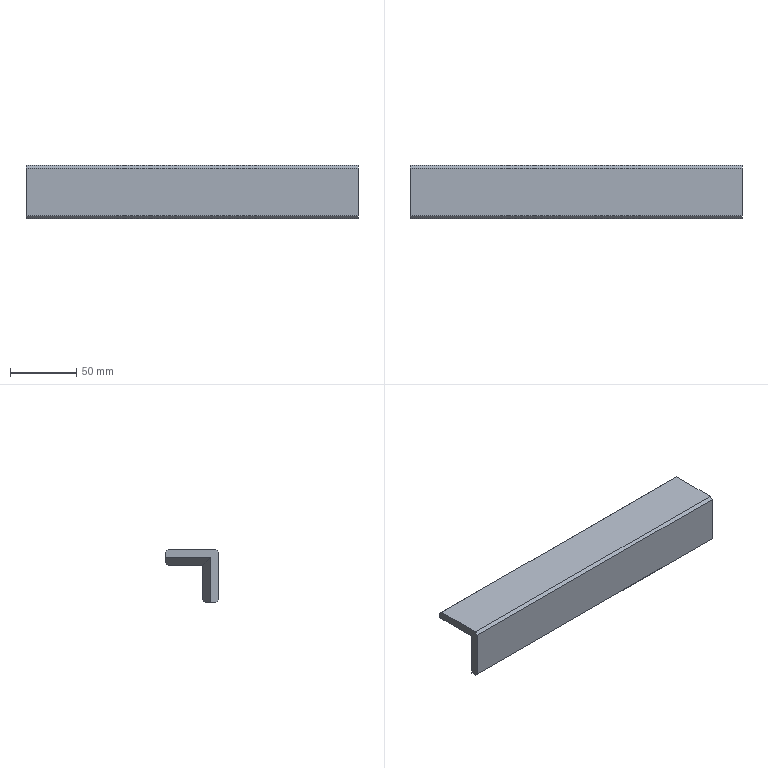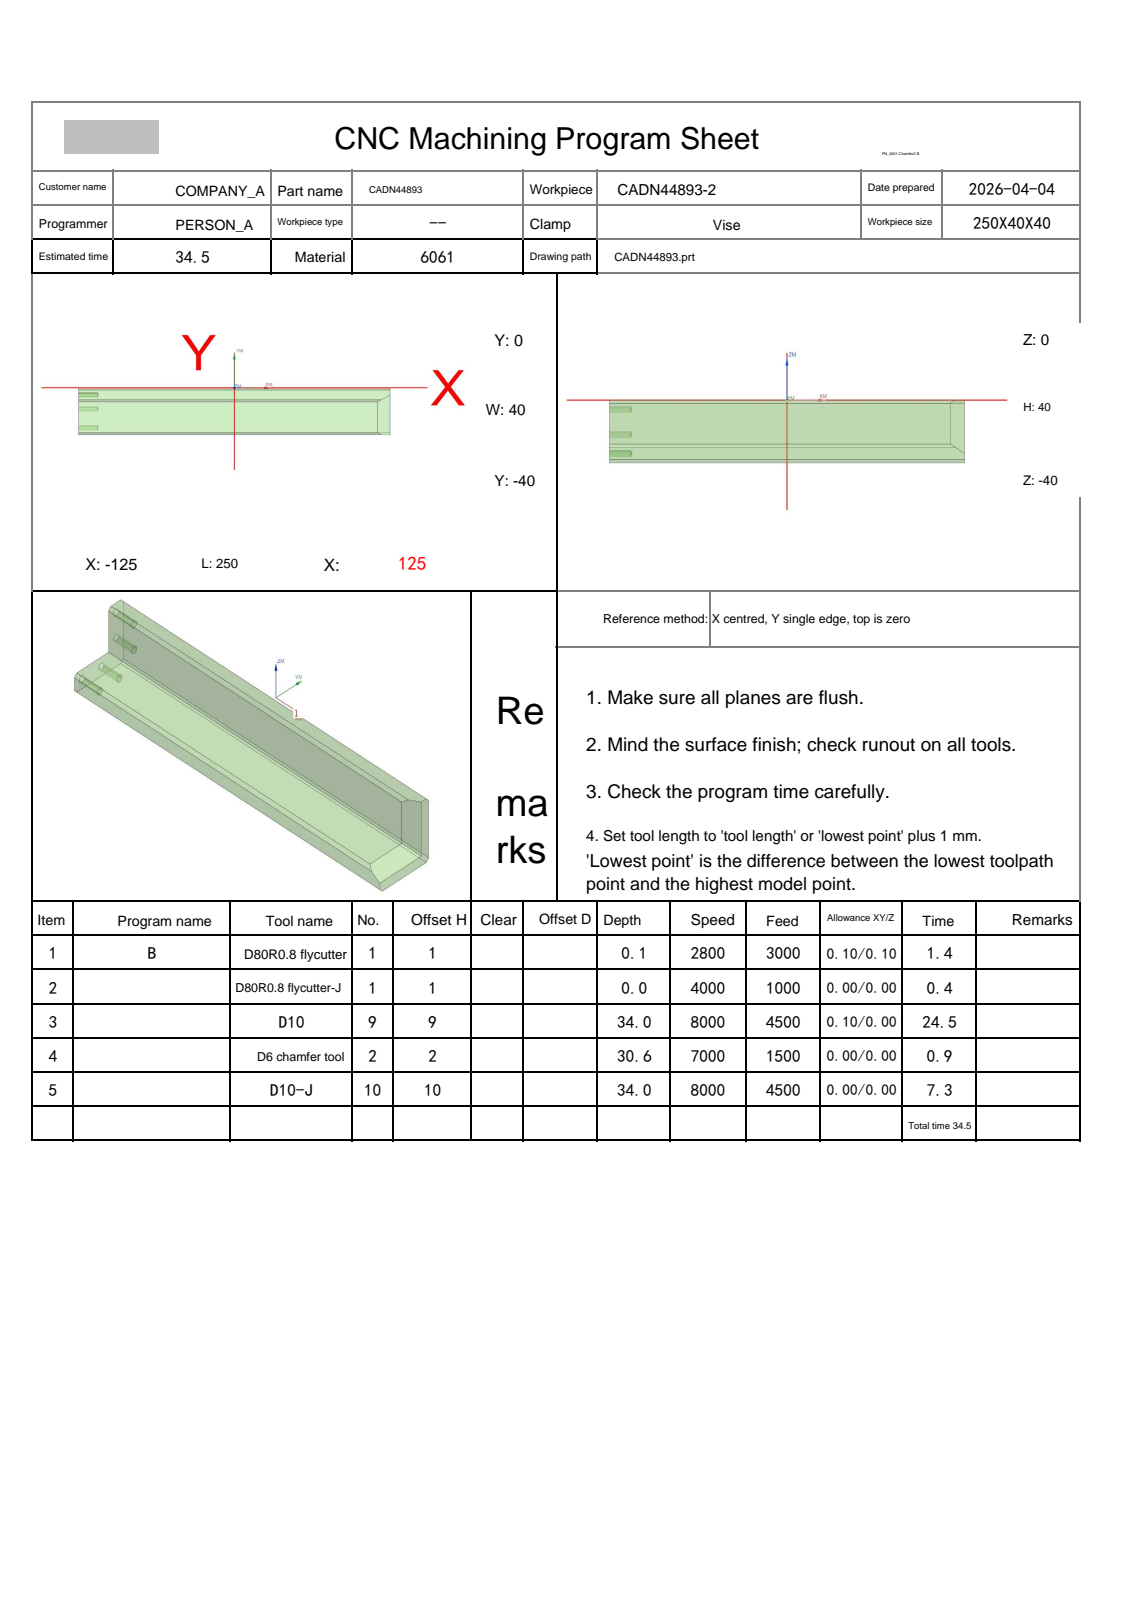NC program | NX | posted by the shop | part box 250 x 40 x 40 mm
Lines 109 to 1286 of 8932:
N3 T09 M06
(D10  D=10. R=0. H=09 ce=0.10 di=0.10)
G00 G90 G54 X8.423 Y-52.151 M03 S8000
G43 H09 Z14.5
M08
Z.702
G01 Z-.498 F4000.
Y-50.
G03 X1.423 Y-43. I-7. J0.0
G01 X-125.08
Y-42.864
Y-17.796
Y-17.039
Y-16.914
Y-15.638
X-118.08 Y-15.64
X117.385
G03 X120.127 Y-14.871 I-.016 J5.333
G01 X127.977 Y-10.161
G03 X129.233 Y-8.844 I-3.041 J4.158
X130.051 Y-6.704 I-4.233 J2.844
G01 X130.074 Y-6.707
X130.147 Y-6.712
X130.131 Y-6.784
Y-9.994
G02 X128.804 Y-11.291 I-5.196 J3.991
G01 X128.698 Y-11.362
X128. Y-11.78
Y-40.08
X123.457
X123.382 Y-40.73
G02 X122.477 Y-43. I-5.03 J.691
G01 X-.563
G02 X-1.375 Y-42.582 I.001 J1.
G01 X-5.778 Y-36.418
G03 X-6.591 Y-36. I-.813 J-.582
G01 X-117.083
G02 X-118.08 Y-35.003 I.003 J1.
G01 Y-23.636
G02 X-117.083 Y-22.64 I1. J-.003
G01 X117.396
G03 X119.806 Y-22.397 I-.026 J12.333
G01 X120. Y-22.378
G02 X121. Y-23.374 I0.0 J-1.
G01 Y-32.868
G02 X120.435 Y-33.765 I-1. J.003
G03 X118.047 Y-35.637 I3.022 J-6.314
G02 X117.279 Y-36. I-.771 J.637
G01 X-.913
G02 X-1.619 Y-35.708 I.001 J1.
G01 X-5.534 Y-31.793
G03 X-6.241 Y-31.5 I-.707 J-.707
G01 X-112.584
G02 X-113.58 Y-30.504 I.004 J1.
G01 Y-28.136
G02 X-112.584 Y-27.14 I1. J-.004
G01 X115.504
G02 X116.5 Y-28.136 I-.004 J-1.
G01 Y-30.443
G02 X116.139 Y-31.208 I-1. J.004
G01 X116.066 Y-31.269
G02 X115.43 Y-31.5 I-.639 J.769
G01 X-3.577
X-4.077
G03 X-11.077 Y-38.5 I0.0 J-7.
G01 Y-52.151
Z.702
G00 Z3.
G01 X8.423 F6000.
G00 Z.204
G01 Z-.996 F4000.
Y-50.
G03 X1.423 Y-43. I-7. J0.0
G01 X-125.08
Y-42.864
Y-17.796
Y-17.099
Y-16.914
Y-16.136
X-118.08 Y-16.138
X116.372
X116.447
G03 X119.297 Y-15.37 I0.0 J5.664
G01 X119.698 Y-15.129
X120.127 Y-14.871
X127.625 Y-10.373
X127.977 Y-10.161
G03 X129.233 Y-8.844 I-3.041 J4.158
X130.051 Y-6.704 I-4.233 J2.844
G01 X130.074 Y-6.707
X130.147 Y-6.712
X130.131 Y-6.784
Y-9.994
G02 X128.804 Y-11.291 I-5.196 J3.991
G01 X128.698 Y-11.362
X128.344 Y-11.574
X128. Y-11.78
Y-40.08
X123.457
X123.382 Y-40.73
G02 X122.477 Y-43. I-5.03 J.691
G01 X-3.577
G02 X-4.548 Y-42.238 I0.0 J1.
G01 X-5.89 Y-36.761
G03 X-6.86 Y-36. I-.971 J-.239
G01 X-117.083
G02 X-118.08 Y-35.004 I.004 J1.
G01 Y-24.134
G02 X-117.084 Y-23.138 I1. J-.004
G01 X116.334
X116.447
G03 X119.743 Y-22.702 I0.0 J12.664
G02 X120. Y-22.668 I.257 J-.967
X121. Y-23.665 I0.0 J-1.
G01 Y-32.869
G02 X120.435 Y-33.765 I-1. J.004
G03 X118.046 Y-35.638 I3.021 J-6.314
G02 X117.28 Y-36. I-.77 J.638
G01 X-.913
G02 X-1.619 Y-35.708 I.001 J1.
G01 X-5.534 Y-31.793
G03 X-6.241 Y-31.5 I-.707 J-.707
G01 X-112.584
G02 X-113.58 Y-30.504 I.004 J1.
G01 Y-28.634
G02 X-112.584 Y-27.638 I1. J-.004
G01 X115.504
G02 X116.5 Y-28.634 I-.004 J-1.
G01 Y-30.443
G02 X116.14 Y-31.208 I-1. J.004
G01 X116.066 Y-31.269
G02 X115.431 Y-31.5 I-.639 J.769
G01 X-3.577
X-4.077
G03 X-11.077 Y-38.5 I0.0 J-7.
G01 Y-52.151
Z.204
G00 Z2.502
G01 X8.423 F6000.
G00 Z-.295
G01 Z-1.495 F4000.
Y-50.
G03 X1.423 Y-43. I-7. J0.0
G01 X-125.08
Y-42.864
Y-17.796
Y-17.099
Y-16.914
Y-16.634
X-118.08 Y-16.636
X115.724
G03 X118.466 Y-15.868 I-.016 J5.333
G01 X127.625 Y-10.373
X127.977 Y-10.161
G03 X129.233 Y-8.844 I-3.041 J4.158
X130.051 Y-6.704 I-4.233 J2.844
G01 X130.074 Y-6.707
X130.147 Y-6.712
X130.131 Y-6.784
Y-9.994
G02 X128.804 Y-11.291 I-5.196 J3.991
G01 X128.698 Y-11.362
X128. Y-11.78
Y-40.08
X123.457
X123.382 Y-40.73
G02 X122.477 Y-43. I-5.03 J.691
G01 X-3.577
G02 X-4.548 Y-42.238 I0.0 J1.
G01 X-5.89 Y-36.761
G03 X-6.86 Y-36. I-.971 J-.239
G01 X-117.084
G02 X-118.08 Y-35.004 I.004 J1.
G01 Y-24.632
G02 X-117.084 Y-23.636 I1. J-.004
G01 X115.735
G03 X119.682 Y-22.979 I-.026 J12.333
G02 X120. Y-22.927 I.318 J-.948
X121. Y-23.923 I0.0 J-1.
G01 Y-32.869
G02 X120.435 Y-33.765 I-1. J.004
G03 X118.046 Y-35.638 I3.021 J-6.314
G02 X117.28 Y-36. I-.77 J.638
G01 X-.913
G02 X-1.619 Y-35.708 I.001 J1.
G01 X-5.534 Y-31.793
G03 X-6.241 Y-31.5 I-.707 J-.707
G01 X-112.584
G02 X-113.58 Y-30.505 I.005 J1.
G01 Y-29.132
G02 X-112.584 Y-28.136 I1. J-.005
G01 X115.505
G02 X116.5 Y-29.132 I-.005 J-1.
G01 Y-30.443
G02 X116.14 Y-31.207 I-1. J.005
G01 X116.066 Y-31.269
G02 X115.431 Y-31.5 I-.639 J.769
G01 X-3.577
X-4.077
G03 X-11.077 Y-38.5 I0.0 J-7.
G01 Y-52.151
Z-.295
G00 Z2.004
G01 X8.423 F6000.
G00 Z-.793
G01 Z-1.993 F4000.
Y-50.
G03 X1.423 Y-43. I-7. J0.0
G01 X-125.08
Y-42.864
Y-18.499
Y-17.796
Y-17.099
X-118.08 Y-17.1
X115.
G03 X117.636 Y-16.366 I-.006 J5.125
G01 X118.466 Y-15.868
X127.625 Y-10.373
X127.977 Y-10.161
G03 X129.233 Y-8.844 I-3.041 J4.158
X130.051 Y-6.704 I-4.233 J2.844
G01 X130.074 Y-6.707
X130.147 Y-6.712
X130.131 Y-6.784
Y-9.994
G02 X128.804 Y-11.291 I-5.196 J3.991
G01 X128.698 Y-11.362
X128.344 Y-11.574
X128. Y-11.78
Y-40.08
X123.457
X123.382 Y-40.73
G02 X122.477 Y-43. I-5.03 J.691
G01 X-3.577
G02 X-4.548 Y-42.238 I0.0 J1.
G01 X-5.89 Y-36.761
G03 X-6.86 Y-36. I-.971 J-.239
G01 X-117.084
G02 X-118.08 Y-35.004 I.004 J1.
G01 Y-25.095
G02 X-117.084 Y-24.1 I1. J-.004
G01 X115.004
G03 X119.622 Y-23.181 I-.011 J12.125
G02 X120. Y-23.107 I.378 J-.926
X121. Y-24.103 I0.0 J-1.
G01 Y-32.869
G02 X120.436 Y-33.765 I-1. J.004
G03 X118.046 Y-35.638 I3.021 J-6.315
G02 X117.28 Y-36. I-.77 J.638
G01 X-.913
G02 X-1.619 Y-35.708 I.001 J1.
G01 X-5.534 Y-31.793
G03 X-6.241 Y-31.5 I-.707 J-.707
G01 X-112.585
G02 X-113.58 Y-30.505 I.005 J1.
G01 Y-29.595
G02 X-112.585 Y-28.6 I1. J-.005
G01 X115.008
G03 X115.476 Y-28.593 I-.015 J16.625
G01 X115.5 Y-28.592
G02 X116.5 Y-29.588 I0.0 J-1.
G01 Y-30.444
G02 X116.14 Y-31.207 I-1. J.005
G01 X116.065 Y-31.269
G02 X115.431 Y-31.5 I-.639 J.769
G01 X-3.577
X-4.077
G03 X-11.077 Y-38.5 I0.0 J-7.
G01 Y-52.151
Z-.793
G00 Z1.505
G01 X8.423 F6000.
G00 Z-1.291
G01 Z-2.491 F4000.
Y-50.
G03 X1.423 Y-43. I-7. J0.0
G01 X-125.08
Y-42.864
Y-18.5
Y-17.796
Y-17.099
X-118.08 Y-17.1
X115.
G03 X116.948 Y-16.713 I0.0 J5.1
X117.636 Y-16.366 I-1.948 J4.713
G01 X118.126 Y-16.072
X118.466 Y-15.868
X127.625 Y-10.372
X127.977 Y-10.161
G03 X129.233 Y-8.844 I-3.041 J4.158
X130.051 Y-6.704 I-4.233 J2.844
G01 X130.074 Y-6.707
X130.147 Y-6.712
X130.131 Y-6.784
Y-9.994
G02 X128.804 Y-11.291 I-5.196 J3.991
G01 X128.698 Y-11.362
X128.344 Y-11.574
X128. Y-11.78
Y-40.08
X123.457
X123.382 Y-40.73
G02 X122.477 Y-43. I-5.03 J.691
G01 X-3.577
G02 X-4.548 Y-42.238 I0.0 J1.
G01 X-5.89 Y-36.761
G03 X-6.86 Y-36. I-.971 J-.239
G01 X-117.084
G02 X-118.08 Y-35.005 I.005 J1.
G01 Y-25.095
G02 X-117.084 Y-24.1 I1. J-.005
G01 X115.
G03 X119.622 Y-23.182 I0.0 J12.1
G02 X120. Y-23.108 I.378 J-.926
X121. Y-24.104 I0.0 J-1.
G01 Y-32.869
G02 X120.436 Y-33.765 I-1. J.005
G03 X118.046 Y-35.638 I3.021 J-6.315
G02 X117.281 Y-36. I-.77 J.638
G01 X-.913
G02 X-1.619 Y-35.708 I.001 J1.
G01 X-5.534 Y-31.793
G03 X-6.241 Y-31.5 I-.707 J-.707
G01 X-112.585
G02 X-113.58 Y-30.505 I.005 J1.
G01 Y-29.595
G02 X-112.585 Y-28.6 I1. J-.005
G01 X115.
G03 X115.476 Y-28.593 I0.0 J16.6
G01 X115.5
G02 X116.5 Y-29.588 I0.0 J-1.
G01 Y-30.444
G02 X116.14 Y-31.207 I-1. J.005
G01 X116.065 Y-31.269
G02 X115.432 Y-31.5 I-.639 J.769
G01 X-3.577
X-4.077
G03 X-11.077 Y-38.5 I0.0 J-7.
G01 Y-52.151
Z-1.291
G00 Z1.007
G01 X8.423 F6000.
G00 Z-1.789
G01 Z-2.989 F4000.
Y-50.
G03 X1.423 Y-43. I-7. J0.0
G01 X-125.08
Y-42.864
Y-18.5
Y-17.796
Y-17.099
X-118.08 Y-17.1
X115.
G03 X116.948 Y-16.713 I0.0 J5.1
X117.636 Y-16.366 I-1.948 J4.713
G01 X118.466 Y-15.868
X118.857 Y-15.633
X119.249 Y-15.398
X127.626 Y-10.372
X127.977 Y-10.161
G03 X129.233 Y-8.844 I-3.041 J4.158
X130.051 Y-6.704 I-4.233 J2.844
G01 X130.074 Y-6.707
X130.147 Y-6.712
X130.131 Y-6.784
Y-9.994
G02 X128.804 Y-11.291 I-5.196 J3.991
G01 X128.698 Y-11.362
X128.344 Y-11.574
X128. Y-11.78
Y-40.08
X123.457
X123.382 Y-40.73
G02 X122.477 Y-43. I-5.03 J.691
G01 X-3.577
G02 X-4.548 Y-42.238 I0.0 J1.
G01 X-5.89 Y-36.761
G03 X-6.86 Y-36. I-.971 J-.239
G01 X-117.085
G02 X-118.08 Y-35.005 I.005 J1.
G01 Y-25.095
G02 X-117.085 Y-24.1 I1. J-.005
G01 X115.
G03 X119.623 Y-23.182 I0.0 J12.1
G02 X120. Y-23.108 I.377 J-.926
X121. Y-24.103 I0.0 J-1.
G01 Y-32.87
G02 X120.436 Y-33.765 I-1. J.005
G03 X118.046 Y-35.638 I3.02 J-6.315
G02 X117.281 Y-36. I-.77 J.638
G01 X-.913
G02 X-1.619 Y-35.708 I.001 J1.
G01 X-5.534 Y-31.793
G03 X-6.241 Y-31.5 I-.707 J-.707
G01 X-112.585
G02 X-113.58 Y-30.505 I.005 J1.
G01 Y-29.595
G02 X-112.585 Y-28.6 I1. J-.005
G01 X115.
G03 X115.477 Y-28.593 I0.0 J16.6
G01 X115.5
G02 X116.5 Y-29.588 I0.0 J-1.
G01 Y-30.444
G02 X116.14 Y-31.207 I-1. J.005
G01 X116.065 Y-31.27
G02 X115.432 Y-31.5 I-.638 J.77
G01 X-3.577
X-4.077
G03 X-11.077 Y-38.5 I0.0 J-7.
G01 Y-52.151
Z-1.789
G00 Z.509
G01 X8.423 F6000.
G00 Z-2.288
G01 Z-3.488 F4000.
Y-50.
G03 X1.423 Y-43. I-7. J0.0
G01 X-125.08
Y-42.864
Y-17.796
Y-17.1
X-118.08
X115.
G03 X116.948 Y-16.713 I0.0 J5.1
X117.636 Y-16.366 I-1.948 J4.713
G01 X127.626 Y-10.372
X127.977 Y-10.161
G03 X129.233 Y-8.844 I-3.041 J4.158
X130.051 Y-6.704 I-4.233 J2.844
G01 X130.074 Y-6.707
X130.147 Y-6.712
X130.131 Y-6.784
Y-9.994
G02 X128.804 Y-11.291 I-5.196 J3.991
G01 X128.698 Y-11.362
X128.344 Y-11.574
X128. Y-11.78
Y-40.08
X123.457
X123.382 Y-40.73
G02 X122.477 Y-43. I-5.03 J.691
G01 X-3.577
G02 X-4.548 Y-42.238 I0.0 J1.
G01 X-5.89 Y-36.761
G03 X-6.86 Y-36. I-.971 J-.239
G01 X-117.085
G02 X-118.08 Y-35.005 I.005 J1.
G01 Y-25.095
G02 X-117.085 Y-24.1 I1. J-.005
G01 X115.
G03 X119.623 Y-23.182 I0.0 J12.1
G02 X120. Y-23.108 I.377 J-.926
X121. Y-24.103 I0.0 J-1.
G01 Y-32.87
G02 X120.436 Y-33.765 I-1. J.005
G03 X118.046 Y-35.639 I3.02 J-6.315
G02 X117.281 Y-36. I-.77 J.639
G01 X-.913
G02 X-1.619 Y-35.708 I.001 J1.
G01 X-5.534 Y-31.793
G03 X-6.241 Y-31.5 I-.707 J-.707
G01 X-112.585
G02 X-113.58 Y-30.506 I.006 J1.
G01 Y-29.594
G02 X-112.585 Y-28.6 I1. J-.006
G01 X115.
G03 X115.477 Y-28.593 I0.0 J16.6
G01 X115.5
G02 X116.5 Y-29.587 I0.0 J-1.
G01 Y-30.444
G02 X116.141 Y-31.207 I-1. J.006
G01 X116.065 Y-31.27
G02 X115.432 Y-31.5 I-.638 J.77
G01 X-3.577
X-4.077
G03 X-11.077 Y-38.5 I0.0 J-7.
G01 Y-52.151
Z-2.288
G00 Z.011
G01 X8.423 F6000.
G00 Z-2.786
G01 Z-3.986 F4000.
Y-50.
G03 X1.423 Y-43. I-7. J0.0
G01 X-125.08
Y-42.864
Y-18.5
Y-17.796
Y-17.099
X-118.08 Y-17.1
X115.
G03 X117.624 Y-16.373 I0.0 J5.1
G01 X127.626 Y-10.372
X127.977 Y-10.161
G03 X129.233 Y-8.844 I-3.041 J4.158
X130.051 Y-6.704 I-4.233 J2.844
G01 X130.074 Y-6.707
X130.147 Y-6.712
X130.131 Y-6.784
Y-9.994
G02 X128.804 Y-11.291 I-5.196 J3.991
G01 X128.698 Y-11.362
X128.344 Y-11.574
X128. Y-11.78
Y-40.08
X123.457
X123.382 Y-40.73
G02 X122.477 Y-43. I-5.03 J.691
G01 X-3.577
G02 X-4.548 Y-42.238 I0.0 J1.
G01 X-5.89 Y-36.761
G03 X-6.86 Y-36. I-.971 J-.239
G01 X-117.085
G02 X-118.08 Y-35.005 I.005 J1.
G01 Y-25.095
G02 X-117.085 Y-24.1 I1. J-.005
G01 X115.
G03 X119.623 Y-23.182 I0.0 J12.1
G02 X120. Y-23.108 I.377 J-.926
X121. Y-24.103 I0.0 J-1.
G01 Y-32.87
G02 X120.437 Y-33.765 I-1. J.005
G03 X118.045 Y-35.639 I3.02 J-6.315
G02 X117.281 Y-36. I-.769 J.639
G01 X-.913
G02 X-1.619 Y-35.708 I.001 J1.
G01 X-5.534 Y-31.793
G03 X-6.241 Y-31.5 I-.707 J-.707
G01 X-112.586
G02 X-113.58 Y-30.506 I.006 J1.
G01 Y-29.594
G02 X-112.586 Y-28.6 I1. J-.006
G01 X115.
G03 X115.477 Y-28.593 I0.0 J16.6
G01 X115.5
G02 X116.5 Y-29.587 I0.0 J-1.
G01 Y-30.445
G02 X116.141 Y-31.207 I-1. J.006
G01 X116.065 Y-31.27
G02 X115.432 Y-31.5 I-.638 J.77
G01 X-3.577
X-4.077
G03 X-11.077 Y-38.5 I0.0 J-7.
G01 Y-52.151
Z-2.786
G00 Z-.488
G01 X8.423 F6000.
G00 Z-3.284
G01 Z-4.484 F4000.
Y-50.
G03 X1.423 Y-43. I-7. J0.0
G01 X-125.08
Y-42.864
Y-18.5
Y-17.796
Y-17.099
X-118.08 Y-17.1
X115.
G03 X117.624 Y-16.373 I0.0 J5.1
G01 X127.977 Y-10.161
G03 X129.233 Y-8.844 I-3.041 J4.158
X130.051 Y-6.704 I-4.233 J2.844
G01 X130.074 Y-6.707
X130.147 Y-6.712
X130.131 Y-6.784
Y-9.994
G02 X128.804 Y-11.291 I-5.196 J3.991
G01 X128.698 Y-11.362
X128.344 Y-11.574
X128. Y-11.78
Y-40.08
X123.457
X123.382 Y-40.73
G02 X122.477 Y-43. I-5.03 J.691
G01 X-3.577
G02 X-4.548 Y-42.238 I0.0 J1.
G01 X-5.89 Y-36.761
G03 X-6.86 Y-36. I-.971 J-.239
G01 X-117.085
G02 X-118.08 Y-35.006 I.006 J1.
G01 Y-25.094
G02 X-117.085 Y-24.1 I1. J-.006
G01 X115.
G03 X119.623 Y-23.182 I0.0 J12.1
G02 X120. Y-23.108 I.377 J-.926
X121. Y-24.103 I0.0 J-1.
G01 Y-32.87
G02 X120.437 Y-33.764 I-1. J.006
G03 X118.045 Y-35.639 I3.02 J-6.315
G02 X117.282 Y-36. I-.769 J.639
G01 X-.913
G02 X-1.619 Y-35.708 I.001 J1.
G01 X-5.534 Y-31.793
G03 X-6.241 Y-31.5 I-.707 J-.707
G01 X-112.586
G02 X-113.58 Y-30.506 I.006 J1.
G01 Y-29.594
G02 X-112.586 Y-28.6 I1. J-.006
G01 X115.
G03 X115.477 Y-28.593 I0.0 J16.6
G01 X115.5
G02 X116.5 Y-29.587 I0.0 J-1.
G01 Y-30.445
G02 X116.141 Y-31.206 I-1. J.006
G01 X116.064 Y-31.27
G02 X115.432 Y-31.5 I-.638 J.77
G01 X-3.577
X-4.077
G03 X-11.077 Y-38.5 I0.0 J-7.
G01 Y-52.151
Z-3.284
G00 Z-.986
G01 X8.423 F6000.
G00 Z-3.782
G01 Z-4.982 F4000.
Y-50.
G03 X1.423 Y-43. I-7. J0.0
G01 X-125.08
Y-42.864
Y-17.796
Y-17.099
X-118.08 Y-17.1
X115.
G03 X117.624 Y-16.373 I0.0 J5.1
G01 X127.627 Y-10.371
X127.977 Y-10.161
G03 X129.233 Y-8.845 I-3.041 J4.158
X130.051 Y-6.704 I-4.233 J2.845
G01 X130.074 Y-6.707
X130.147 Y-6.712
X130.131 Y-6.784
Y-9.994
G02 X128.804 Y-11.291 I-5.196 J3.991
G01 X128.698 Y-11.362
X128.344 Y-11.574
X128. Y-11.78
Y-40.08
X123.457
X123.382 Y-40.73
G02 X122.477 Y-43. I-5.03 J.691
G01 X-3.577
G02 X-4.548 Y-42.238 I0.0 J1.
G01 X-5.89 Y-36.761
G03 X-6.86 Y-36. I-.971 J-.239
G01 X-117.086
G02 X-118.08 Y-35.006 I.006 J1.
G01 Y-25.094
G02 X-117.086 Y-24.1 I1. J-.006
G01 X115.
G03 X119.623 Y-23.182 I0.0 J12.1
G02 X120. Y-23.108 I.377 J-.926
X121. Y-24.102 I0.0 J-1.
G01 Y-32.871
G02 X120.437 Y-33.764 I-1. J.006
G03 X118.045 Y-35.639 I3.02 J-6.315
G02 X117.282 Y-36. I-.769 J.639
G01 X-.913
G02 X-1.619 Y-35.708 I.001 J1.
G01 X-5.534 Y-31.793
G03 X-6.241 Y-31.5 I-.707 J-.707
G01 X-112.586
G02 X-113.58 Y-30.506 I.006 J1.
G01 Y-29.594
G02 X-112.586 Y-28.6 I1. J-.006
G01 X115.
G03 X115.478 Y-28.593 I0.0 J16.6
G01 X115.5
G02 X116.5 Y-29.587 I0.0 J-1.
G01 Y-30.445
G02 X116.141 Y-31.206 I-1. J.006
G01 X116.064 Y-31.27
G02 X115.433 Y-31.5 I-.638 J.77
G01 X-3.577
X-4.077
G03 X-11.077 Y-38.5 I0.0 J-7.
G01 Y-52.151
Z-3.782
G00 Z-1.484
G01 X8.423 F6000.
G00 Z-4.28
G01 Z-5.48 F4000.
Y-50.
G03 X1.423 Y-43. I-7. J0.0
G01 X-125.08
Y-42.864
Y-17.796
Y-17.099
X-118.08 Y-17.1
X115.
G03 X117.624 Y-16.373 I0.0 J5.1
G01 X127.627 Y-10.371
X127.977 Y-10.161
G03 X129.233 Y-8.845 I-3.041 J4.158
X130.051 Y-6.704 I-4.233 J2.845
G01 X130.074 Y-6.707
X130.147 Y-6.712
X130.131 Y-6.784
Y-9.994
G02 X128.804 Y-11.291 I-5.196 J3.991
G01 X128.698 Y-11.362
X128.344 Y-11.574
X128. Y-11.78
Y-40.08
X123.457
X123.382 Y-40.73
G02 X122.477 Y-43. I-5.03 J.691
G01 X-3.577
G02 X-4.548 Y-42.238 I0.0 J1.
G01 X-5.89 Y-36.761
G03 X-6.86 Y-36. I-.971 J-.239
G01 X-117.086
G02 X-118.08 Y-35.006 I.006 J1.
G01 Y-25.094
G02 X-117.086 Y-24.1 I1. J-.006
G01 X115.
G03 X119.624 Y-23.182 I0.0 J12.1
G02 X120. Y-23.108 I.376 J-.926
X121. Y-24.102 I0.0 J-1.
G01 Y-32.871
G02 X120.437 Y-33.764 I-1. J.006
G03 X118.045 Y-35.639 I3.019 J-6.315
G02 X117.282 Y-36. I-.769 J.639
G01 X-.913
G02 X-1.619 Y-35.708 I.001 J1.
G01 X-5.534 Y-31.793
G03 X-6.241 Y-31.5 I-.707 J-.707
G01 X-112.586
G02 X-113.58 Y-30.506 I.006 J1.
G01 Y-29.594
G02 X-112.586 Y-28.6 I1. J-.006
G01 X115.
G03 X115.478 Y-28.593 I0.0 J16.6
G01 X115.5
G02 X116.5 Y-29.587 I0.0 J-1.
G01 Y-30.445
G02 X116.141 Y-31.206 I-1. J.006
G01 X116.064 Y-31.27
G02 X115.433 Y-31.5 I-.638 J.77
G01 X-3.577
X-4.077
G03 X-11.077 Y-38.5 I0.0 J-7.
G01 Y-52.151
Z-4.28
G00 Z-1.982
G01 X8.423 F6000.
G00 Z-4.779
G01 Z-5.979 F4000.
Y-50.
G03 X1.423 Y-43. I-7. J0.0
G01 X-125.08
Y-42.864
Y-17.796
Y-17.1
X-118.08
X115.
G03 X117.624 Y-16.373 I0.0 J5.1
G01 X127.627 Y-10.371
X127.977 Y-10.161
G03 X129.233 Y-8.845 I-3.041 J4.158
X130.051 Y-6.704 I-4.233 J2.845
G01 X130.074 Y-6.707
X130.147 Y-6.712
X130.131 Y-6.784
Y-9.994
G02 X128.804 Y-11.291 I-5.196 J3.991
G01 X128.698 Y-11.362
X128.344 Y-11.574
X128. Y-11.78
Y-40.08
X123.457
X123.382 Y-40.73
G02 X122.477 Y-43. I-5.03 J.691
G01 X-3.577
G02 X-4.548 Y-42.238 I0.0 J1.
G01 X-5.89 Y-36.761
G03 X-6.86 Y-36. I-.971 J-.239
G01 X-117.086
G02 X-118.08 Y-35.006 I.006 J1.
G01 Y-25.094
G02 X-117.086 Y-24.1 I1. J-.006
G01 X115.
G03 X119.624 Y-23.182 I0.0 J12.1
G02 X120. Y-23.108 I.376 J-.927
X121. Y-24.102 I0.0 J-1.
G01 Y-32.871
G02 X120.437 Y-33.764 I-1. J.006
G03 X118.045 Y-35.639 I3.019 J-6.315
G02 X117.282 Y-36. I-.769 J.639
G01 X-.913
G02 X-1.619 Y-35.708 I.001 J1.
G01 X-5.534 Y-31.793
G03 X-6.241 Y-31.5 I-.707 J-.707
G01 X-112.586
G02 X-113.58 Y-30.507 I.007 J1.
G01 Y-29.593
G02 X-112.586 Y-28.6 I1. J-.007
G01 X115.
G03 X115.478 Y-28.593 I0.0 J16.6
G01 X115.5
G02 X116.5 Y-29.586 I0.0 J-1.
G01 Y-30.445
G02 X116.141 Y-31.206 I-1. J.007
G01 X116.064 Y-31.27
G02 X115.433 Y-31.5 I-.638 J.77
G01 X-3.577
X-4.077
G03 X-11.077 Y-38.5 I0.0 J-7.
G01 Y-52.151
Z-4.779
G00 Z-2.48
G01 X8.423 F6000.
G00 Z-5.277
G01 Z-6.477 F4000.
Y-50.
G03 X1.423 Y-43. I-7. J0.0
G01 X-125.08
Y-42.864
Y-17.796
Y-17.099
X-118.08 Y-17.1
X115.
G03 X117.624 Y-16.373 I0.0 J5.1
G01 X127.627 Y-10.371
X127.977 Y-10.161
G03 X129.233 Y-8.845 I-3.041 J4.158
X130.051 Y-6.704 I-4.233 J2.845
G01 X130.074 Y-6.707
X130.147 Y-6.712
X130.131 Y-6.784
Y-9.994
G02 X128.804 Y-11.291 I-5.196 J3.991
G01 X128.698 Y-11.362
X128.344 Y-11.574
X128. Y-11.78
Y-40.08
X123.457
X123.382 Y-40.73
G02 X122.477 Y-43. I-5.03 J.691
G01 X-3.577
G02 X-4.548 Y-42.238 I0.0 J1.
G01 X-5.89 Y-36.761
G03 X-6.86 Y-36. I-.971 J-.239
G01 X-117.086
G02 X-118.08 Y-35.006 I.006 J1.
G01 Y-25.094
G02 X-117.086 Y-24.1 I1. J-.006
G01 X115.
G03 X119.624 Y-23.182 I0.0 J12.1
G02 X120. Y-23.108 I.376 J-.927
X121. Y-24.102 I0.0 J-1.
G01 Y-32.871
G02 X120.437 Y-33.764 I-1. J.006
G03 X118.045 Y-35.64 I3.019 J-6.315
G02 X117.282 Y-36. I-.769 J.64
G01 X-.913
G02 X-1.619 Y-35.708 I.001 J1.
G01 X-5.534 Y-31.793
G03 X-6.241 Y-31.5 I-.707 J-.707
G01 X-112.587
G02 X-113.58 Y-30.507 I.007 J1.
G01 Y-29.593
G02 X-112.587 Y-28.6 I1. J-.007
G01 X115.
G03 X115.478 Y-28.593 I0.0 J16.6
G01 X115.5
G02 X116.5 Y-29.586 I0.0 J-1.
G01 Y-30.446
G02 X116.141 Y-31.206 I-1. J.007
G01 X116.064 Y-31.271
G02 X115.433 Y-31.5 I-.637 J.77
G01 X-3.577
X-4.077
G03 X-11.077 Y-38.5 I0.0 J-7.
G01 Y-52.151
Z-5.277
G00 Z-2.979
G01 X8.423 F6000.
G00 Z-5.775
G01 Z-6.975 F4000.
Y-50.
G03 X1.423 Y-43. I-7. J0.0
G01 X-125.08
Y-42.864
Y-17.796
Y-17.099
X-118.08 Y-17.1
X115.
G03 X117.624 Y-16.373 I0.0 J5.1
G01 X127.628 Y-10.371
X127.977 Y-10.161
G03 X129.233 Y-8.845 I-3.041 J4.158
X130.051 Y-6.704 I-4.233 J2.845
G01 X130.074 Y-6.707
X130.147 Y-6.712
X130.131 Y-6.784
Y-9.994
G02 X128.804 Y-11.291 I-5.196 J3.991
G01 X128.698 Y-11.362
X128.344 Y-11.574
X128. Y-11.78
Y-40.08
X123.457
X123.382 Y-40.73
G02 X122.477 Y-43. I-5.03 J.691
G01 X-3.577
G02 X-4.548 Y-42.238 I0.0 J1.
G01 X-5.89 Y-36.761
G03 X-6.86 Y-36. I-.971 J-.239
G01 X-117.086
G02 X-118.08 Y-35.007 I.007 J1.
G01 Y-25.093
G02 X-117.086 Y-24.1 I1. J-.007
G01 X115.
G03 X119.624 Y-23.182 I0.0 J12.1
G02 X120. Y-23.108 I.376 J-.927
X121. Y-24.102 I0.0 J-1.
G01 Y-32.871
G02 X120.438 Y-33.764 I-1. J.007
G03 X118.045 Y-35.64 I3.019 J-6.316
G02 X117.283 Y-36. I-.769 J.64
G01 X-.913
G02 X-1.619 Y-35.708 I.001 J1.
G01 X-5.534 Y-31.793
G03 X-6.241 Y-31.5 I-.707 J-.707
G01 X-112.587
G02 X-113.58 Y-30.507 I.007 J1.
G01 Y-29.593
G02 X-112.587 Y-28.6 I1. J-.007
G01 X115.
G03 X115.478 Y-28.593 I0.0 J16.6
G01 X115.5
G02 X116.5 Y-29.586 I0.0 J-1.
G01 Y-30.446
G02 X116.142 Y-31.206 I-1. J.007
G01 X116.064 Y-31.271
G02 X115.433 Y-31.5 I-.637 J.771
G01 X-3.577
X-4.077
G03 X-11.077 Y-38.5 I0.0 J-7.
G01 Y-52.151
Z-5.775
G00 Z-3.477
G01 X8.423 F6000.
G00 Z-6.273
G01 Z-7.473 F4000.
Y-50.
G03 X1.423 Y-43. I-7. J0.0
G01 X-125.08
Y-42.864
Y-18.5
Y-17.796
Y-17.099
X-118.08 Y-17.1
X115.
G03 X117.624 Y-16.373 I0.0 J5.1
G01 X127.628 Y-10.371
X127.977 Y-10.161
G03 X129.233 Y-8.845 I-3.041 J4.158
X130.051 Y-6.704 I-4.233 J2.845
G01 X130.074 Y-6.707
X130.147 Y-6.712
X130.131 Y-6.784
Y-9.994
G02 X128.804 Y-11.291 I-5.196 J3.991
G01 X128.698 Y-11.362
X128.344 Y-11.574
X128. Y-11.78
Y-40.08
X123.457
X123.382 Y-40.73
G02 X122.477 Y-43. I-5.03 J.691
G01 X-3.577
G02 X-4.548 Y-42.238 I0.0 J1.
G01 X-5.89 Y-36.761
G03 X-6.86 Y-36. I-.971 J-.239
G01 X-117.087
G02 X-118.08 Y-35.007 I.007 J1.
G01 Y-25.093
G02 X-117.087 Y-24.1 I1. J-.007
G01 X115.
G03 X119.624 Y-23.181 I0.0 J12.1
G02 X120. Y-23.108 I.376 J-.927
X121. Y-24.101 I0.0 J-1.
G01 Y-32.872
G02 X120.438 Y-33.764 I-1. J.007
G03 X118.045 Y-35.64 I3.019 J-6.316
G02 X117.283 Y-36. I-.769 J.64
G01 X-.913
G02 X-1.619 Y-35.708 I.001 J1.
G01 X-5.534 Y-31.793
G03 X-6.241 Y-31.5 I-.707 J-.707
G01 X-112.587
G02 X-113.58 Y-30.507 I.007 J1.
G01 Y-29.593
G02 X-112.587 Y-28.6 I1. J-.007
G01 X115.
G03 X115.478 Y-28.593 I0.0 J16.6
G01 X115.5
G02 X116.5 Y-29.586 I0.0 J-1.
G01 Y-30.446
G02 X116.142 Y-31.206 I-1. J.007
G01 X116.064 Y-31.271
G02 X115.434 Y-31.5 I-.637 J.771
G01 X-3.577
X-4.077
G03 X-11.077 Y-38.5 I0.0 J-7.
G01 Y-52.151
Z-6.273
G00 Z-3.975
G01 X8.423 F6000.
G00 Z-6.771
G01 Z-7.971 F4000.
Y-50.
G03 X1.423 Y-43. I-7. J0.0
G01 X-125.08
Y-42.864
Y-17.796
Y-17.1
X-118.08
X115.
G03 X117.624 Y-16.373 I0.0 J5.1
G01 X127.628 Y-10.371
X127.977 Y-10.161
G03 X129.233 Y-8.845 I-3.041 J4.158
X130.051 Y-6.704 I-4.233 J2.845
G01 X130.074 Y-6.707
X130.147 Y-6.712
X130.131 Y-6.784
Y-9.994
G02 X128.804 Y-11.291 I-5.196 J3.991
G01 X128.698 Y-11.362
X128.344 Y-11.574
X128. Y-11.78
Y-40.08
X123.457
X123.382 Y-40.73
G02 X122.477 Y-43. I-5.03 J.691
G01 X-3.577
G02 X-4.548 Y-42.238 I0.0 J1.
G01 X-5.89 Y-36.761
G03 X-6.86 Y-36. I-.971 J-.239
G01 X-117.087
G02 X-118.08 Y-35.007 I.007 J1.
G01 Y-25.093
G02 X-117.087 Y-24.1 I1. J-.007
G01 X115.
G03 X119.624 Y-23.181 I0.0 J12.1
G02 X120. Y-23.108 I.376 J-.927
X121. Y-24.101 I0.0 J-1.
G01 Y-32.872
G02 X120.438 Y-33.764 I-1. J.007
G03 X118.045 Y-35.64 I3.019 J-6.316
G02 X117.283 Y-36. I-.768 J.64
G01 X-.913
G02 X-1.619 Y-35.708 I.001 J1.
G01 X-5.534 Y-31.793
G03 X-6.241 Y-31.5 I-.707 J-.707
G01 X-112.587
G02 X-113.58 Y-30.507 I.007 J1.
G01 Y-29.593
G02 X-112.587 Y-28.6 I1. J-.007
G01 X115.
G03 X115.479 Y-28.593 I0.0 J16.6
G01 X115.5
G02 X116.5 Y-29.586 I0.0 J-1.
G01 Y-30.446
G02 X116.142 Y-31.206 I-1. J.007
G01 X116.064 Y-31.271
G02 X115.434 Y-31.5 I-.637 J.771
G01 X-3.577
X-4.077
G03 X-11.077 Y-38.5 I0.0 J-7.
G01 Y-52.151
Z-6.771
G00 Z-4.473
G01 X8.423 F6000.
G00 Z-7.27
G01 Z-8.47 F4000.
Y-50.
G03 X1.423 Y-43. I-7. J0.0
G01 X-125.08
Y-42.864
Y-17.796
Y-17.099
X-118.08 Y-17.1
X115.
G03 X117.624 Y-16.373 I0.0 J5.1
G01 X127.628 Y-10.371
X127.977 Y-10.161
G03 X129.233 Y-8.845 I-3.041 J4.158
X130.051 Y-6.704 I-4.233 J2.845
G01 X130.074 Y-6.707
X130.147 Y-6.712
X130.131 Y-6.784
Y-9.994
G02 X128.804 Y-11.291 I-5.196 J3.991
G01 X128.698 Y-11.362
X128.344 Y-11.574
X128. Y-11.78
Y-40.08
X123.457
X123.382 Y-40.73
G02 X122.477 Y-43. I-5.03 J.691
G01 X-3.577
G02 X-4.548 Y-42.238 I0.0 J1.
G01 X-5.89 Y-36.761
G03 X-6.86 Y-36. I-.971 J-.239
G01 X-117.087
G02 X-118.08 Y-35.007 I.007 J1.
G01 Y-25.093
G02 X-117.087 Y-24.1 I1. J-.007
G01 X115.
G03 X119.625 Y-23.181 I0.0 J12.1
G02 X120. Y-23.108 I.375 J-.927
X121. Y-24.101 I0.0 J-1.
G01 Y-32.872
G02 X120.438 Y-33.764 I-1. J.007
G03 X118.044 Y-35.64 I3.019 J-6.316
G02 X117.283 Y-36. I-.768 J.64
G01 X-.913
G02 X-1.619 Y-35.708 I.001 J1.
G01 X-5.534 Y-31.793
G03 X-6.241 Y-31.5 I-.707 J-.707
G01 X-112.587
G02 X-113.58 Y-30.507 I.007 J1.
G01 Y-29.593
G02 X-112.587 Y-28.6 I1. J-.007
G01 X115.
G03 X115.479 Y-28.593 I0.0 J16.6
G01 X115.5
G02 X116.5 Y-29.585 I0.0 J-1.
G01 Y-30.446
G02 X116.142 Y-31.206 I-1. J.007
G01 X116.063 Y-31.271
G02 X115.434 Y-31.5 I-.637 J.771
G01 X-3.577
X-4.077
G03 X-11.077 Y-38.5 I0.0 J-7.
G01 Y-52.151
Z-7.27
G00 Z-4.971
G01 X8.423 F6000.
G00 Z-7.768
G01 Z-8.968 F4000.
Y-50.
G03 X1.423 Y-43. I-7. J0.0
G01 X-125.08
Y-42.864
Y-18.5
Y-17.796
Y-17.099
X-118.08 Y-17.1
X115.
G03 X117.624 Y-16.373 I0.0 J5.1
G01 X127.977 Y-10.161
G03 X129.233 Y-8.845 I-3.041 J4.158
X130.051 Y-6.704 I-4.233 J2.845
G01 X130.074 Y-6.707
X130.147 Y-6.712
X130.131 Y-6.784
Y-9.994
G02 X128.804 Y-11.291 I-5.196 J3.991
G01 X128.698 Y-11.362
X128.344 Y-11.574
X128. Y-11.78
Y-40.08
X123.457
X123.382 Y-40.73
G02 X122.477 Y-43. I-5.03 J.691
G01 X-3.577
G02 X-4.548 Y-42.238 I0.0 J1.
G01 X-5.89 Y-36.761
G03 X-6.86 Y-36. I-.971 J-.239
G01 X-117.087
G02 X-118.08 Y-35.007 I.007 J1.
G01 Y-25.093
G02 X-117.087 Y-24.1 I1. J-.007
G01 X115.